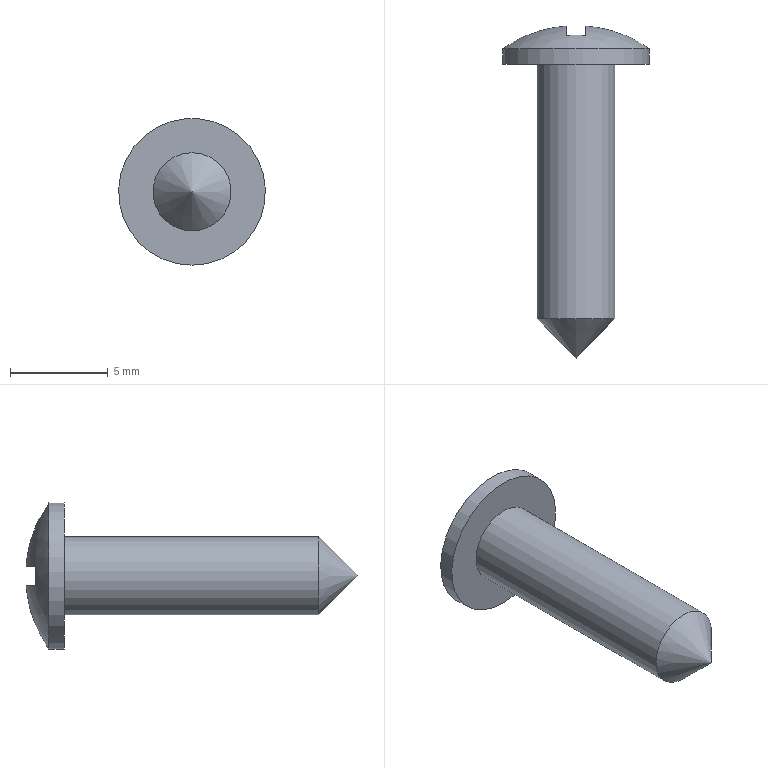Part | STEP file | ZG0415 | 1 solid | 18 faces | box 7.5 x 16.961 x 7.5 mm | volume 227.201 mm3 | plane 14 | cylinder 2 | cone 1 | sphere 1 | commonest cylinder face diameters 4 x1 7.5 x1